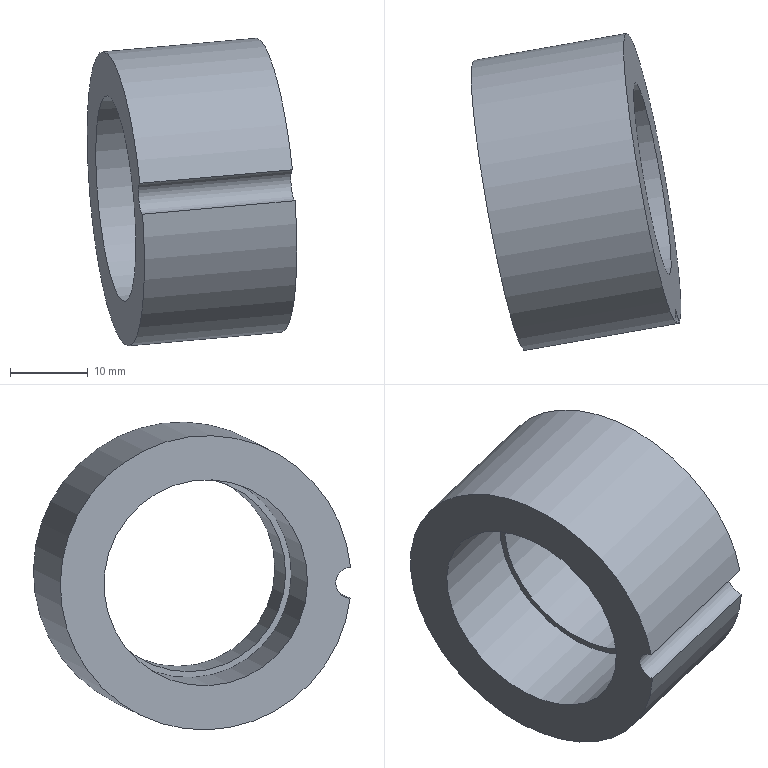Part | NX | features solid 2 | 1 solid | 7 faces | box 26.982 x 40.811 x 39.599 mm | volume 11932 mm3 | cylinder 4 | plane 3 | commonest cylinder face diameters 4 x1 25.1 x1 26.6 x1 38 x1
STEP:
#1=CARTESIAN_POINT('',(1479.257,537.547,6.151));
#2=VERTEX_POINT('',#1);
#3=CARTESIAN_POINT('',(1498.879,541.007,7.894));
#4=VERTEX_POINT('',#3);
#5=CARTESIAN_POINT('',(1489.068,539.277,7.022));
#6=DIRECTION('',(0.9811,0.173,0.08716));
#7=VECTOR('',#6,1000.);
#8=LINE('',#5,#7);
#9=EDGE_CURVE('',#2,#4,#8,.T.);
#10=ORIENTED_EDGE('',*,*,#9,.F.);
#11=CARTESIAN_POINT('',(1478.914,537.487,10.13));
#12=VERTEX_POINT('',#11);
#13=CARTESIAN_POINT('',(1475.805,556.124,8.14));
#14=DIRECTION('',(0.9811,0.173,0.08716));
#15=DIRECTION('',(0.1736,-0.9848,0.));
#16=AXIS2_PLACEMENT_3D('',#13,#14,#15);
#17=CIRCLE('',#16,19.);
#18=EDGE_CURVE('',#2,#12,#17,.T.);
#19=ORIENTED_EDGE('',*,*,#18,.T.);
#20=CARTESIAN_POINT('',(1498.536,540.946,11.873));
#21=VERTEX_POINT('',#20);
#22=CARTESIAN_POINT('',(1488.725,539.216,11.001));
#23=DIRECTION('',(0.9811,0.173,0.08716));
#24=VECTOR('',#23,1000.);
#25=LINE('',#22,#24);
#26=EDGE_CURVE('',#21,#12,#25,.F.);
#27=ORIENTED_EDGE('',*,*,#26,.F.);
#28=CARTESIAN_POINT('',(1495.426,559.584,9.883));
#29=DIRECTION('',(0.9811,0.173,0.08716));
#30=DIRECTION('',(0.1736,-0.9848,0.));
#31=AXIS2_PLACEMENT_3D('',#28,#29,#30);
#32=CIRCLE('',#31,19.);
#33=EDGE_CURVE('',#4,#21,#32,.T.);
#34=ORIENTED_EDGE('',*,*,#33,.F.);
#35=EDGE_LOOP('',(#10,#19,#27,#34));
#36=FACE_BOUND('',#35,.T.);
#37=CARTESIAN_POINT('',(1475.805,556.124,8.14));
#38=DIRECTION('',(0.9811,0.173,0.08716));
#39=DIRECTION('',(0.1736,-0.9848,0.));
#40=AXIS2_PLACEMENT_3D('',#37,#38,#39);
#41=CYLINDRICAL_SURFACE('',#40,19.);
#42=ADVANCED_FACE('',(#36),#41,.T.);
#43=CARTESIAN_POINT('',(1478.114,543.027,8.14));
#44=VERTEX_POINT('',#43);
#45=CARTESIAN_POINT('',(1475.805,556.124,8.14));
#46=DIRECTION('',(0.9811,0.173,0.08716));
#47=DIRECTION('',(0.1736,-0.9848,0.));
#48=AXIS2_PLACEMENT_3D('',#45,#46,#47);
#49=CIRCLE('',#48,13.3);
#50=EDGE_CURVE('',#44,#44,#49,.T.);
#51=ORIENTED_EDGE('',*,*,#50,.T.);
#52=EDGE_LOOP('',(#51));
#53=FACE_BOUND('',#52,.T.);
#54=ORIENTED_EDGE('',*,*,#18,.F.);
#55=CARTESIAN_POINT('',(1479.104,537.413,8.14));
#56=DIRECTION('',(0.9811,0.173,0.08716));
#57=DIRECTION('',(0.1736,-0.9848,0.));
#58=AXIS2_PLACEMENT_3D('',#55,#56,#57);
#59=CIRCLE('',#58,2.);
#60=EDGE_CURVE('',#2,#12,#59,.T.);
#61=ORIENTED_EDGE('',*,*,#60,.T.);
#62=EDGE_LOOP('',(#54,#61));
#63=FACE_BOUND('',#62,.T.);
#64=CARTESIAN_POINT('',(1475.805,556.124,8.14));
#65=DIRECTION('',(0.9811,0.173,0.08716));
#66=DIRECTION('',(0.1736,-0.9848,0.));
#67=AXIS2_PLACEMENT_3D('',#64,#65,#66);
#68=PLANE('',#67);
#69=ADVANCED_FACE('',(#53,#63),#68,.F.);
#70=CARTESIAN_POINT('',(1497.605,547.225,9.883));
#71=VERTEX_POINT('',#70);
#72=CARTESIAN_POINT('',(1495.426,559.584,9.883));
#73=DIRECTION('',(0.9811,0.173,0.08716));
#74=DIRECTION('',(0.1736,-0.9848,0.));
#75=AXIS2_PLACEMENT_3D('',#72,#73,#74);
#76=CIRCLE('',#75,12.55);
#77=EDGE_CURVE('',#71,#71,#76,.T.);
#78=ORIENTED_EDGE('',*,*,#77,.F.);
#79=EDGE_LOOP('',(#78));
#80=FACE_BOUND('',#79,.T.);
#81=CARTESIAN_POINT('',(1498.725,540.873,9.883));
#82=DIRECTION('',(0.9811,0.173,0.08716));
#83=DIRECTION('',(0.1736,-0.9848,0.));
#84=AXIS2_PLACEMENT_3D('',#81,#82,#83);
#85=CIRCLE('',#84,2.);
#86=EDGE_CURVE('',#4,#21,#85,.T.);
#87=ORIENTED_EDGE('',*,*,#86,.F.);
#88=ORIENTED_EDGE('',*,*,#33,.T.);
#89=EDGE_LOOP('',(#87,#88));
#90=FACE_BOUND('',#89,.T.);
#91=CARTESIAN_POINT('',(1495.426,559.584,9.883));
#92=DIRECTION('',(0.9811,0.173,0.08716));
#93=DIRECTION('',(0.1736,-0.9848,0.));
#94=AXIS2_PLACEMENT_3D('',#91,#92,#93);
#95=PLANE('',#94);
#96=ADVANCED_FACE('',(#80,#90),#95,.T.);
#97=ORIENTED_EDGE('',*,*,#50,.F.);
#98=EDGE_LOOP('',(#97));
#99=FACE_BOUND('',#98,.T.);
#100=CARTESIAN_POINT('',(1489.887,545.102,9.186));
#101=VERTEX_POINT('',#100);
#102=CARTESIAN_POINT('',(1487.578,558.2,9.186));
#103=DIRECTION('',(0.9811,0.173,0.08716));
#104=DIRECTION('',(0.1736,-0.9848,0.));
#105=AXIS2_PLACEMENT_3D('',#102,#103,#104);
#106=CIRCLE('',#105,13.3);
#107=EDGE_CURVE('',#101,#101,#106,.T.);
#108=ORIENTED_EDGE('',*,*,#107,.T.);
#109=EDGE_LOOP('',(#108));
#110=FACE_BOUND('',#109,.T.);
#111=CARTESIAN_POINT('',(1475.805,556.124,8.14));
#112=DIRECTION('',(0.9811,0.173,0.08716));
#113=DIRECTION('',(0.1736,-0.9848,0.));
#114=AXIS2_PLACEMENT_3D('',#111,#112,#113);
#115=CYLINDRICAL_SURFACE('',#114,13.3);
#116=ADVANCED_FACE('',(#99,#110),#115,.F.);
#117=CARTESIAN_POINT('',(1489.757,545.841,9.186));
#118=VERTEX_POINT('',#117);
#119=CARTESIAN_POINT('',(1487.578,558.2,9.186));
#120=DIRECTION('',(0.9811,0.173,0.08716));
#121=DIRECTION('',(0.1736,-0.9848,0.));
#122=AXIS2_PLACEMENT_3D('',#119,#120,#121);
#123=CIRCLE('',#122,12.55);
#124=EDGE_CURVE('',#118,#118,#123,.T.);
#125=ORIENTED_EDGE('',*,*,#124,.T.);
#126=EDGE_LOOP('',(#125));
#127=FACE_BOUND('',#126,.T.);
#128=ORIENTED_EDGE('',*,*,#107,.F.);
#129=EDGE_LOOP('',(#128));
#130=FACE_BOUND('',#129,.T.);
#131=CARTESIAN_POINT('',(1487.578,558.2,9.186));
#132=DIRECTION('',(0.9811,0.173,0.08716));
#133=DIRECTION('',(0.1736,-0.9848,0.));
#134=AXIS2_PLACEMENT_3D('',#131,#132,#133);
#135=PLANE('',#134);
#136=ADVANCED_FACE('',(#127,#130),#135,.F.);
#137=ORIENTED_EDGE('',*,*,#9,.T.);
#138=ORIENTED_EDGE('',*,*,#86,.T.);
#139=ORIENTED_EDGE('',*,*,#26,.T.);
#140=ORIENTED_EDGE('',*,*,#60,.F.);
#141=EDGE_LOOP('',(#137,#138,#139,#140));
#142=FACE_BOUND('',#141,.T.);
#143=CARTESIAN_POINT('',(1479.104,537.413,8.14));
#144=DIRECTION('',(0.9811,0.173,0.08716));
#145=DIRECTION('',(0.1736,-0.9848,0.));
#146=AXIS2_PLACEMENT_3D('',#143,#144,#145);
#147=CYLINDRICAL_SURFACE('',#146,2.);
#148=ADVANCED_FACE('',(#142),#147,.F.);
#149=ORIENTED_EDGE('',*,*,#77,.T.);
#150=EDGE_LOOP('',(#149));
#151=FACE_BOUND('',#150,.T.);
#152=ORIENTED_EDGE('',*,*,#124,.F.);
#153=EDGE_LOOP('',(#152));
#154=FACE_BOUND('',#153,.T.);
#155=CARTESIAN_POINT('',(1475.805,556.124,8.14));
#156=DIRECTION('',(0.9811,0.173,0.08716));
#157=DIRECTION('',(0.1736,-0.9848,0.));
#158=AXIS2_PLACEMENT_3D('',#155,#156,#157);
#159=CYLINDRICAL_SURFACE('',#158,12.55);
#160=ADVANCED_FACE('',(#151,#154),#159,.F.);
#161=CLOSED_SHELL('',(#42,#69,#96,#116,#136,#148,#160));
#162=MANIFOLD_SOLID_BREP('',#161);
#163=(LENGTH_UNIT()NAMED_UNIT(*)SI_UNIT(.MILLI.,.METRE.));
#164=UNCERTAINTY_MEASURE_WITH_UNIT(LENGTH_MEASURE(0.00001),#163,'','');
#165=(NAMED_UNIT(*)PLANE_ANGLE_UNIT()SI_UNIT($,.RADIAN.));
#166=(NAMED_UNIT(*)SI_UNIT($,.STERADIAN.)SOLID_ANGLE_UNIT());
#167=(GEOMETRIC_REPRESENTATION_CONTEXT(3)GLOBAL_UNCERTAINTY_ASSIGNED_CONTEXT((#164))GLOBAL_UNIT_ASSIGNED_CONTEXT((#163,#165,#166))REPRESENTATION_CONTEXT('',''));
#168=ADVANCED_BREP_SHAPE_REPRESENTATION('',(#162),#167);